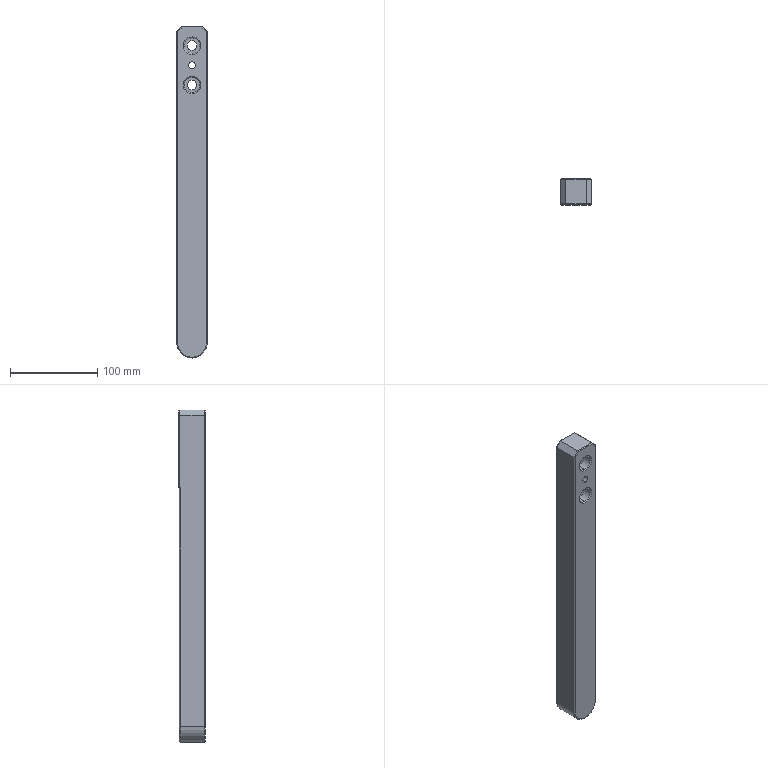Part | Creo | 1 solid | 44 faces | box 35 x 30 x 380 mm | volume 377331 mm3 | plane 23 | cylinder 11 | cone 10 | commonest cylinder face diameters 11 x4 18 x4 8 x2 35 x1
STEP:
#1=CARTESIAN_POINT('',(0.,0.,0.));
#2=DIRECTION('',(0.,0.,1.));
#3=DIRECTION('',(1.,0.,0.));
#4=AXIS2_PLACEMENT_3D('',#1,#2,#3);
#5=CARTESIAN_POINT('',(129.,-219.,0.5));
#6=VERTEX_POINT('',#5);
#7=CARTESIAN_POINT('',(130.,-220.,0.5));
#8=VERTEX_POINT('',#7);
#9=CARTESIAN_POINT('',(129.,-219.,0.5));
#10=DIRECTION('',(0.7071,-0.7071,0.));
#11=VECTOR('',#10,1.414);
#12=LINE('',#9,#11);
#13=EDGE_CURVE('',#6,#8,#12,.T.);
#14=ORIENTED_EDGE('',*,*,#13,.F.);
#15=CARTESIAN_POINT('',(96.,-219.,0.5));
#16=VERTEX_POINT('',#15);
#17=CARTESIAN_POINT('',(129.,-219.,0.5));
#18=DIRECTION('',(-1.,0.,0.));
#19=VECTOR('',#18,33.);
#20=LINE('',#17,#19);
#21=EDGE_CURVE('',#6,#16,#20,.T.);
#22=ORIENTED_EDGE('',*,*,#21,.T.);
#23=CARTESIAN_POINT('',(95.,-220.,0.5));
#24=VERTEX_POINT('',#23);
#25=CARTESIAN_POINT('',(95.,-220.,0.5));
#26=DIRECTION('',(0.7071,0.7071,0.));
#27=VECTOR('',#26,1.414);
#28=LINE('',#25,#27);
#29=EDGE_CURVE('',#24,#16,#28,.T.);
#30=ORIENTED_EDGE('',*,*,#29,.F.);
#31=CARTESIAN_POINT('',(95.,-220.5,0.5));
#32=VERTEX_POINT('',#31);
#33=CARTESIAN_POINT('',(95.,-220.,0.5));
#34=DIRECTION('',(0.,-1.,0.));
#35=VECTOR('',#34,0.5);
#36=LINE('',#33,#35);
#37=EDGE_CURVE('',#24,#32,#36,.T.);
#38=ORIENTED_EDGE('',*,*,#37,.T.);
#39=CARTESIAN_POINT('',(96.,-219.5,0.5));
#40=VERTEX_POINT('',#39);
#41=CARTESIAN_POINT('',(96.,-219.5,0.5));
#42=DIRECTION('',(-0.7071,-0.7071,0.));
#43=VECTOR('',#42,1.414);
#44=LINE('',#41,#43);
#45=EDGE_CURVE('',#40,#32,#44,.T.);
#46=ORIENTED_EDGE('',*,*,#45,.F.);
#47=CARTESIAN_POINT('',(129.,-219.5,0.5));
#48=VERTEX_POINT('',#47);
#49=CARTESIAN_POINT('',(96.,-219.5,0.5));
#50=DIRECTION('',(1.,0.,0.));
#51=VECTOR('',#50,33.);
#52=LINE('',#49,#51);
#53=EDGE_CURVE('',#40,#48,#52,.T.);
#54=ORIENTED_EDGE('',*,*,#53,.T.);
#55=CARTESIAN_POINT('',(130.,-220.5,0.5));
#56=VERTEX_POINT('',#55);
#57=CARTESIAN_POINT('',(130.,-220.5,0.5));
#58=DIRECTION('',(-0.7071,0.7071,0.));
#59=VECTOR('',#58,1.414);
#60=LINE('',#57,#59);
#61=EDGE_CURVE('',#56,#48,#60,.T.);
#62=ORIENTED_EDGE('',*,*,#61,.F.);
#63=CARTESIAN_POINT('',(130.,-220.,0.5));
#64=DIRECTION('',(0.,-1.,0.));
#65=VECTOR('',#64,0.5);
#66=LINE('',#63,#65);
#67=EDGE_CURVE('',#8,#56,#66,.T.);
#68=ORIENTED_EDGE('',*,*,#67,.F.);
#69=EDGE_LOOP('',(#14,#22,#30,#38,#46,#54,#62,#68));
#70=FACE_OUTER_BOUND('',#69,.F.);
#71=CARTESIAN_POINT('',(0.,-7.,0.5));
#72=DIRECTION('',(0.,0.,-1.));
#73=DIRECTION('',(1.,0.,0.));
#74=AXIS2_PLACEMENT_3D('',#71,#72,#73);
#75=PLANE('',#74);
#76=ADVANCED_FACE('',(#70),#75,.T.);
#77=CARTESIAN_POINT('',(130.,-220.,83.5));
#78=VERTEX_POINT('',#77);
#79=CARTESIAN_POINT('',(130.,-220.,83.5));
#80=DIRECTION('',(0.,0.,-1.));
#81=VECTOR('',#80,83.);
#82=LINE('',#79,#81);
#83=EDGE_CURVE('',#78,#8,#82,.T.);
#84=ORIENTED_EDGE('',*,*,#83,.F.);
#85=CARTESIAN_POINT('',(129.,-219.,83.086));
#86=VERTEX_POINT('',#85);
#87=CARTESIAN_POINT('',(129.,-219.,83.086));
#88=DIRECTION('',(0.6786,-0.6786,0.2811));
#89=VECTOR('',#88,1.474);
#90=LINE('',#87,#89);
#91=EDGE_CURVE('',#86,#78,#90,.T.);
#92=ORIENTED_EDGE('',*,*,#91,.F.);
#93=CARTESIAN_POINT('',(129.,-219.,0.5));
#94=DIRECTION('',(0.,0.,1.));
#95=VECTOR('',#94,82.586);
#96=LINE('',#93,#95);
#97=EDGE_CURVE('',#6,#86,#96,.T.);
#98=ORIENTED_EDGE('',*,*,#97,.F.);
#99=ORIENTED_EDGE('',*,*,#13,.T.);
#100=EDGE_LOOP('',(#84,#92,#98,#99));
#101=FACE_OUTER_BOUND('',#100,.F.);
#102=CARTESIAN_POINT('',(129.,-219.,0.));
#103=DIRECTION('',(-0.7071,-0.7071,0.));
#104=DIRECTION('',(0.,0.,-1.));
#105=AXIS2_PLACEMENT_3D('',#102,#103,#104);
#106=PLANE('',#105);
#107=ADVANCED_FACE('',(#101),#106,.F.);
#108=CARTESIAN_POINT('',(130.,-220.5,-273.));
#109=VERTEX_POINT('',#108);
#110=CARTESIAN_POINT('',(130.,-248.,-273.));
#111=VERTEX_POINT('',#110);
#112=CARTESIAN_POINT('',(130.,-220.5,-273.));
#113=DIRECTION('',(0.,-1.,0.));
#114=VECTOR('',#113,27.5);
#115=LINE('',#112,#114);
#116=EDGE_CURVE('',#109,#111,#115,.T.);
#117=ORIENTED_EDGE('',*,*,#116,.T.);
#118=CARTESIAN_POINT('',(130.,-248.,83.5));
#119=VERTEX_POINT('',#118);
#120=CARTESIAN_POINT('',(130.,-248.,-273.));
#121=DIRECTION('',(0.,0.,1.));
#122=VECTOR('',#121,356.5);
#123=LINE('',#120,#122);
#124=EDGE_CURVE('',#111,#119,#123,.T.);
#125=ORIENTED_EDGE('',*,*,#124,.T.);
#126=CARTESIAN_POINT('',(130.,-248.,83.5));
#127=DIRECTION('',(0.,1.,0.));
#128=VECTOR('',#127,28.);
#129=LINE('',#126,#128);
#130=EDGE_CURVE('',#119,#78,#129,.T.);
#131=ORIENTED_EDGE('',*,*,#130,.T.);
#132=ORIENTED_EDGE('',*,*,#83,.T.);
#133=ORIENTED_EDGE('',*,*,#67,.T.);
#134=CARTESIAN_POINT('',(130.,-220.5,0.5));
#135=DIRECTION('',(0.,0.,-1.));
#136=VECTOR('',#135,273.5);
#137=LINE('',#134,#136);
#138=EDGE_CURVE('',#56,#109,#137,.T.);
#139=ORIENTED_EDGE('',*,*,#138,.T.);
#140=EDGE_LOOP('',(#117,#125,#131,#132,#133,#139));
#141=FACE_OUTER_BOUND('',#140,.F.);
#142=CARTESIAN_POINT('',(130.,-249.,79.5));
#143=DIRECTION('',(1.,0.,0.));
#144=DIRECTION('',(0.,0.,-1.));
#145=AXIS2_PLACEMENT_3D('',#142,#143,#144);
#146=PLANE('',#145);
#147=ADVANCED_FACE('',(#141),#146,.T.);
#148=CARTESIAN_POINT('',(95.,-248.,-273.));
#149=VERTEX_POINT('',#148);
#150=CARTESIAN_POINT('',(95.,-220.5,-273.));
#151=VERTEX_POINT('',#150);
#152=CARTESIAN_POINT('',(95.,-248.,-273.));
#153=DIRECTION('',(0.,1.,0.));
#154=VECTOR('',#153,27.5);
#155=LINE('',#152,#154);
#156=EDGE_CURVE('',#149,#151,#155,.T.);
#157=ORIENTED_EDGE('',*,*,#156,.F.);
#158=CARTESIAN_POINT('',(112.5,-248.,-290.5));
#159=VERTEX_POINT('',#158);
#160=CARTESIAN_POINT('',(112.5,-248.,-273.));
#161=DIRECTION('',(0.,-1.,0.));
#162=DIRECTION('',(-1.,0.,0.));
#163=AXIS2_PLACEMENT_3D('',#160,#161,#162);
#164=CIRCLE('',#163,17.5);
#165=EDGE_CURVE('',#149,#159,#164,.T.);
#166=ORIENTED_EDGE('',*,*,#165,.T.);
#167=CARTESIAN_POINT('',(112.5,-248.,-273.));
#168=DIRECTION('',(0.,-1.,0.));
#169=DIRECTION('',(0.,0.,-1.));
#170=AXIS2_PLACEMENT_3D('',#167,#168,#169);
#171=CIRCLE('',#170,17.5);
#172=EDGE_CURVE('',#159,#111,#171,.T.);
#173=ORIENTED_EDGE('',*,*,#172,.T.);
#174=ORIENTED_EDGE('',*,*,#116,.F.);
#175=CARTESIAN_POINT('',(112.5,-220.5,-290.5));
#176=VERTEX_POINT('',#175);
#177=CARTESIAN_POINT('',(112.5,-220.5,-273.));
#178=DIRECTION('',(0.,1.,0.));
#179=DIRECTION('',(1.,0.,0.));
#180=AXIS2_PLACEMENT_3D('',#177,#178,#179);
#181=CIRCLE('',#180,17.5);
#182=EDGE_CURVE('',#109,#176,#181,.T.);
#183=ORIENTED_EDGE('',*,*,#182,.T.);
#184=CARTESIAN_POINT('',(112.5,-220.5,-273.));
#185=DIRECTION('',(0.,1.,0.));
#186=DIRECTION('',(0.,0.,-1.));
#187=AXIS2_PLACEMENT_3D('',#184,#185,#186);
#188=CIRCLE('',#187,17.5);
#189=EDGE_CURVE('',#176,#151,#188,.T.);
#190=ORIENTED_EDGE('',*,*,#189,.T.);
#191=EDGE_LOOP('',(#157,#166,#173,#174,#183,#190));
#192=FACE_OUTER_BOUND('',#191,.F.);
#193=CARTESIAN_POINT('',(112.5,-249.,-273.));
#194=DIRECTION('',(0.,1.,0.));
#195=DIRECTION('',(0.,0.,-1.));
#196=AXIS2_PLACEMENT_3D('',#193,#194,#195);
#197=CYLINDRICAL_SURFACE('',#196,17.5);
#198=ADVANCED_FACE('',(#192),#197,.T.);
#199=CARTESIAN_POINT('',(95.,-220.,83.5));
#200=VERTEX_POINT('',#199);
#201=CARTESIAN_POINT('',(95.,-220.,0.5));
#202=DIRECTION('',(0.,0.,1.));
#203=VECTOR('',#202,83.);
#204=LINE('',#201,#203);
#205=EDGE_CURVE('',#24,#200,#204,.T.);
#206=ORIENTED_EDGE('',*,*,#205,.T.);
#207=CARTESIAN_POINT('',(95.,-248.,83.5));
#208=VERTEX_POINT('',#207);
#209=CARTESIAN_POINT('',(95.,-220.,83.5));
#210=DIRECTION('',(0.,-1.,0.));
#211=VECTOR('',#210,28.);
#212=LINE('',#209,#211);
#213=EDGE_CURVE('',#200,#208,#212,.T.);
#214=ORIENTED_EDGE('',*,*,#213,.T.);
#215=CARTESIAN_POINT('',(95.,-248.,83.5));
#216=DIRECTION('',(0.,0.,-1.));
#217=VECTOR('',#216,356.5);
#218=LINE('',#215,#217);
#219=EDGE_CURVE('',#208,#149,#218,.T.);
#220=ORIENTED_EDGE('',*,*,#219,.T.);
#221=ORIENTED_EDGE('',*,*,#156,.T.);
#222=CARTESIAN_POINT('',(95.,-220.5,-273.));
#223=DIRECTION('',(0.,0.,1.));
#224=VECTOR('',#223,273.5);
#225=LINE('',#222,#224);
#226=EDGE_CURVE('',#151,#32,#225,.T.);
#227=ORIENTED_EDGE('',*,*,#226,.T.);
#228=ORIENTED_EDGE('',*,*,#37,.F.);
#229=EDGE_LOOP('',(#206,#214,#220,#221,#227,#228));
#230=FACE_OUTER_BOUND('',#229,.F.);
#231=CARTESIAN_POINT('',(95.,-249.,-320.5));
#232=DIRECTION('',(-1.,0.,0.));
#233=DIRECTION('',(0.,0.,1.));
#234=AXIS2_PLACEMENT_3D('',#231,#232,#233);
#235=PLANE('',#234);
#236=ADVANCED_FACE('',(#230),#235,.T.);
#237=ORIENTED_EDGE('',*,*,#29,.T.);
#238=CARTESIAN_POINT('',(96.,-219.,83.086));
#239=VERTEX_POINT('',#238);
#240=CARTESIAN_POINT('',(96.,-219.,83.086));
#241=DIRECTION('',(0.,0.,-1.));
#242=VECTOR('',#241,82.586);
#243=LINE('',#240,#242);
#244=EDGE_CURVE('',#239,#16,#243,.T.);
#245=ORIENTED_EDGE('',*,*,#244,.F.);
#246=CARTESIAN_POINT('',(96.,-219.,83.086));
#247=DIRECTION('',(-0.6786,-0.6786,0.2811));
#248=VECTOR('',#247,1.474);
#249=LINE('',#246,#248);
#250=EDGE_CURVE('',#239,#200,#249,.T.);
#251=ORIENTED_EDGE('',*,*,#250,.T.);
#252=ORIENTED_EDGE('',*,*,#205,.F.);
#253=EDGE_LOOP('',(#237,#245,#251,#252));
#254=FACE_OUTER_BOUND('',#253,.F.);
#255=CARTESIAN_POINT('',(96.,-219.,0.));
#256=DIRECTION('',(0.7071,-0.7071,0.));
#257=DIRECTION('',(0.,0.,1.));
#258=AXIS2_PLACEMENT_3D('',#255,#256,#257);
#259=PLANE('',#258);
#260=ADVANCED_FACE('',(#254),#259,.F.);
#261=ORIENTED_EDGE('',*,*,#21,.F.);
#262=ORIENTED_EDGE('',*,*,#97,.T.);
#263=CARTESIAN_POINT('',(123.586,-219.,88.5));
#264=VERTEX_POINT('',#263);
#265=CARTESIAN_POINT('',(123.586,-219.,88.5));
#266=DIRECTION('',(0.7071,0.,-0.7071));
#267=VECTOR('',#266,7.657);
#268=LINE('',#265,#267);
#269=EDGE_CURVE('',#264,#86,#268,.T.);
#270=ORIENTED_EDGE('',*,*,#269,.F.);
#271=CARTESIAN_POINT('',(101.414,-219.,88.5));
#272=VERTEX_POINT('',#271);
#273=CARTESIAN_POINT('',(123.586,-219.,88.5));
#274=DIRECTION('',(-1.,0.,0.));
#275=VECTOR('',#274,22.172);
#276=LINE('',#273,#275);
#277=EDGE_CURVE('',#264,#272,#276,.T.);
#278=ORIENTED_EDGE('',*,*,#277,.T.);
#279=CARTESIAN_POINT('',(96.,-219.,83.086));
#280=DIRECTION('',(0.7071,0.,0.7071));
#281=VECTOR('',#280,7.657);
#282=LINE('',#279,#281);
#283=EDGE_CURVE('',#239,#272,#282,.T.);
#284=ORIENTED_EDGE('',*,*,#283,.F.);
#285=ORIENTED_EDGE('',*,*,#244,.T.);
#286=EDGE_LOOP('',(#261,#262,#270,#278,#284,#285));
#287=FACE_OUTER_BOUND('',#286,.F.);
#288=CARTESIAN_POINT('',(112.5,-219.,15.5));
#289=VERTEX_POINT('',#288);
#290=CARTESIAN_POINT('',(112.5,-219.,28.5));
#291=VERTEX_POINT('',#290);
#292=CARTESIAN_POINT('',(112.5,-219.,22.));
#293=DIRECTION('',(0.,-1.,0.));
#294=DIRECTION('',(0.,0.,-1.));
#295=AXIS2_PLACEMENT_3D('',#292,#293,#294);
#296=CIRCLE('',#295,6.5);
#297=EDGE_CURVE('',#289,#291,#296,.T.);
#298=ORIENTED_EDGE('',*,*,#297,.F.);
#299=CARTESIAN_POINT('',(112.5,-219.,22.));
#300=DIRECTION('',(0.,-1.,0.));
#301=DIRECTION('',(0.,0.,1.));
#302=AXIS2_PLACEMENT_3D('',#299,#300,#301);
#303=CIRCLE('',#302,6.5);
#304=EDGE_CURVE('',#291,#289,#303,.T.);
#305=ORIENTED_EDGE('',*,*,#304,.F.);
#306=EDGE_LOOP('',(#298,#305));
#307=FACE_BOUND('',#306,.F.);
#308=CARTESIAN_POINT('',(112.5,-219.,60.5));
#309=VERTEX_POINT('',#308);
#310=CARTESIAN_POINT('',(112.5,-219.,73.5));
#311=VERTEX_POINT('',#310);
#312=CARTESIAN_POINT('',(112.5,-219.,67.));
#313=DIRECTION('',(0.,-1.,0.));
#314=DIRECTION('',(0.,0.,-1.));
#315=AXIS2_PLACEMENT_3D('',#312,#313,#314);
#316=CIRCLE('',#315,6.5);
#317=EDGE_CURVE('',#309,#311,#316,.T.);
#318=ORIENTED_EDGE('',*,*,#317,.F.);
#319=CARTESIAN_POINT('',(112.5,-219.,67.));
#320=DIRECTION('',(0.,-1.,0.));
#321=DIRECTION('',(0.,0.,1.));
#322=AXIS2_PLACEMENT_3D('',#319,#320,#321);
#323=CIRCLE('',#322,6.5);
#324=EDGE_CURVE('',#311,#309,#323,.T.);
#325=ORIENTED_EDGE('',*,*,#324,.F.);
#326=EDGE_LOOP('',(#318,#325));
#327=FACE_BOUND('',#326,.F.);
#328=CARTESIAN_POINT('',(112.5,-219.,40.5));
#329=VERTEX_POINT('',#328);
#330=CARTESIAN_POINT('',(112.5,-219.,48.5));
#331=VERTEX_POINT('',#330);
#332=CARTESIAN_POINT('',(112.5,-219.,44.5));
#333=DIRECTION('',(0.,-1.,0.));
#334=DIRECTION('',(0.,0.,-1.));
#335=AXIS2_PLACEMENT_3D('',#332,#333,#334);
#336=CIRCLE('',#335,4.);
#337=EDGE_CURVE('',#329,#331,#336,.T.);
#338=ORIENTED_EDGE('',*,*,#337,.F.);
#339=CARTESIAN_POINT('',(112.5,-219.,44.5));
#340=DIRECTION('',(0.,-1.,0.));
#341=DIRECTION('',(0.,0.,1.));
#342=AXIS2_PLACEMENT_3D('',#339,#340,#341);
#343=CIRCLE('',#342,4.);
#344=EDGE_CURVE('',#331,#329,#343,.T.);
#345=ORIENTED_EDGE('',*,*,#344,.F.);
#346=EDGE_LOOP('',(#338,#345));
#347=FACE_BOUND('',#346,.F.);
#348=CARTESIAN_POINT('',(0.,-219.,0.));
#349=DIRECTION('',(0.,1.,0.));
#350=DIRECTION('',(0.,0.,1.));
#351=AXIS2_PLACEMENT_3D('',#348,#349,#350);
#352=PLANE('',#351);
#353=ADVANCED_FACE('',(#287,#307,#327,#347),#352,.T.);
#354=ORIENTED_EDGE('',*,*,#337,.T.);
#355=CARTESIAN_POINT('',(112.5,-249.,48.5));
#356=VERTEX_POINT('',#355);
#357=CARTESIAN_POINT('',(112.5,-249.,48.5));
#358=DIRECTION('',(0.,1.,0.));
#359=VECTOR('',#358,30.);
#360=LINE('',#357,#359);
#361=EDGE_CURVE('',#356,#331,#360,.T.);
#362=ORIENTED_EDGE('',*,*,#361,.F.);
#363=CARTESIAN_POINT('',(112.5,-249.,40.5));
#364=VERTEX_POINT('',#363);
#365=CARTESIAN_POINT('',(112.5,-249.,44.5));
#366=DIRECTION('',(0.,1.,0.));
#367=DIRECTION('',(0.,0.,1.));
#368=AXIS2_PLACEMENT_3D('',#365,#366,#367);
#369=CIRCLE('',#368,4.);
#370=EDGE_CURVE('',#356,#364,#369,.T.);
#371=ORIENTED_EDGE('',*,*,#370,.T.);
#372=CARTESIAN_POINT('',(112.5,-249.,40.5));
#373=DIRECTION('',(0.,1.,0.));
#374=VECTOR('',#373,30.);
#375=LINE('',#372,#374);
#376=EDGE_CURVE('',#364,#329,#375,.T.);
#377=ORIENTED_EDGE('',*,*,#376,.T.);
#378=EDGE_LOOP('',(#354,#362,#371,#377));
#379=FACE_OUTER_BOUND('',#378,.F.);
#380=CARTESIAN_POINT('',(112.5,-249.,44.5));
#381=DIRECTION('',(0.,1.,0.));
#382=DIRECTION('',(0.,0.,-1.));
#383=AXIS2_PLACEMENT_3D('',#380,#381,#382);
#384=CYLINDRICAL_SURFACE('',#383,4.);
#385=ADVANCED_FACE('',(#379),#384,.F.);
#386=ORIENTED_EDGE('',*,*,#344,.T.);
#387=ORIENTED_EDGE('',*,*,#376,.F.);
#388=CARTESIAN_POINT('',(112.5,-249.,44.5));
#389=DIRECTION('',(0.,1.,0.));
#390=DIRECTION('',(0.,0.,-1.));
#391=AXIS2_PLACEMENT_3D('',#388,#389,#390);
#392=CIRCLE('',#391,4.);
#393=EDGE_CURVE('',#364,#356,#392,.T.);
#394=ORIENTED_EDGE('',*,*,#393,.T.);
#395=ORIENTED_EDGE('',*,*,#361,.T.);
#396=EDGE_LOOP('',(#386,#387,#394,#395));
#397=FACE_OUTER_BOUND('',#396,.F.);
#398=CARTESIAN_POINT('',(112.5,-249.,44.5));
#399=DIRECTION('',(0.,1.,0.));
#400=DIRECTION('',(0.,0.,-1.));
#401=AXIS2_PLACEMENT_3D('',#398,#399,#400);
#402=CYLINDRICAL_SURFACE('',#401,4.);
#403=ADVANCED_FACE('',(#397),#402,.F.);
#404=CARTESIAN_POINT('',(101.414,-249.,88.5));
#405=VERTEX_POINT('',#404);
#406=CARTESIAN_POINT('',(123.586,-249.,88.5));
#407=VERTEX_POINT('',#406);
#408=CARTESIAN_POINT('',(101.414,-249.,88.5));
#409=DIRECTION('',(1.,0.,0.));
#410=VECTOR('',#409,22.172);
#411=LINE('',#408,#410);
#412=EDGE_CURVE('',#405,#407,#411,.T.);
#413=ORIENTED_EDGE('',*,*,#412,.T.);
#414=CARTESIAN_POINT('',(129.,-249.,83.086));
#415=VERTEX_POINT('',#414);
#416=CARTESIAN_POINT('',(129.,-249.,83.086));
#417=DIRECTION('',(-0.7071,0.,0.7071));
#418=VECTOR('',#417,7.657);
#419=LINE('',#416,#418);
#420=EDGE_CURVE('',#415,#407,#419,.T.);
#421=ORIENTED_EDGE('',*,*,#420,.F.);
#422=CARTESIAN_POINT('',(129.,-249.,-273.));
#423=VERTEX_POINT('',#422);
#424=CARTESIAN_POINT('',(129.,-249.,83.086));
#425=DIRECTION('',(0.,0.,-1.));
#426=VECTOR('',#425,356.086);
#427=LINE('',#424,#426);
#428=EDGE_CURVE('',#415,#423,#427,.T.);
#429=ORIENTED_EDGE('',*,*,#428,.T.);
#430=CARTESIAN_POINT('',(96.,-249.,-273.));
#431=VERTEX_POINT('',#430);
#432=CARTESIAN_POINT('',(112.5,-249.,-273.));
#433=DIRECTION('',(0.,-1.,0.));
#434=DIRECTION('',(-1.,0.,0.));
#435=AXIS2_PLACEMENT_3D('',#432,#433,#434);
#436=CIRCLE('',#435,16.5);
#437=EDGE_CURVE('',#431,#423,#436,.T.);
#438=ORIENTED_EDGE('',*,*,#437,.F.);
#439=CARTESIAN_POINT('',(96.,-249.,83.086));
#440=VERTEX_POINT('',#439);
#441=CARTESIAN_POINT('',(96.,-249.,-273.));
#442=DIRECTION('',(0.,0.,1.));
#443=VECTOR('',#442,356.086);
#444=LINE('',#441,#443);
#445=EDGE_CURVE('',#431,#440,#444,.T.);
#446=ORIENTED_EDGE('',*,*,#445,.T.);
#447=CARTESIAN_POINT('',(101.414,-249.,88.5));
#448=DIRECTION('',(-0.7071,0.,-0.7071));
#449=VECTOR('',#448,7.657);
#450=LINE('',#447,#449);
#451=EDGE_CURVE('',#405,#440,#450,.T.);
#452=ORIENTED_EDGE('',*,*,#451,.F.);
#453=EDGE_LOOP('',(#413,#421,#429,#438,#446,#452));
#454=FACE_OUTER_BOUND('',#453,.F.);
#455=CARTESIAN_POINT('',(112.5,-249.,12.));
#456=VERTEX_POINT('',#455);
#457=CARTESIAN_POINT('',(112.5,-249.,32.));
#458=VERTEX_POINT('',#457);
#459=CARTESIAN_POINT('',(112.5,-249.,22.));
#460=DIRECTION('',(0.,1.,0.));
#461=DIRECTION('',(0.,0.,-1.));
#462=AXIS2_PLACEMENT_3D('',#459,#460,#461);
#463=CIRCLE('',#462,10.);
#464=EDGE_CURVE('',#456,#458,#463,.T.);
#465=ORIENTED_EDGE('',*,*,#464,.F.);
#466=CARTESIAN_POINT('',(112.5,-249.,22.));
#467=DIRECTION('',(0.,1.,0.));
#468=DIRECTION('',(0.,0.,1.));
#469=AXIS2_PLACEMENT_3D('',#466,#467,#468);
#470=CIRCLE('',#469,10.);
#471=EDGE_CURVE('',#458,#456,#470,.T.);
#472=ORIENTED_EDGE('',*,*,#471,.F.);
#473=EDGE_LOOP('',(#465,#472));
#474=FACE_BOUND('',#473,.F.);
#475=CARTESIAN_POINT('',(112.5,-249.,57.));
#476=VERTEX_POINT('',#475);
#477=CARTESIAN_POINT('',(112.5,-249.,77.));
#478=VERTEX_POINT('',#477);
#479=CARTESIAN_POINT('',(112.5,-249.,67.));
#480=DIRECTION('',(0.,1.,0.));
#481=DIRECTION('',(0.,0.,-1.));
#482=AXIS2_PLACEMENT_3D('',#479,#480,#481);
#483=CIRCLE('',#482,10.);
#484=EDGE_CURVE('',#476,#478,#483,.T.);
#485=ORIENTED_EDGE('',*,*,#484,.F.);
#486=CARTESIAN_POINT('',(112.5,-249.,67.));
#487=DIRECTION('',(0.,1.,0.));
#488=DIRECTION('',(0.,0.,1.));
#489=AXIS2_PLACEMENT_3D('',#486,#487,#488);
#490=CIRCLE('',#489,10.);
#491=EDGE_CURVE('',#478,#476,#490,.T.);
#492=ORIENTED_EDGE('',*,*,#491,.F.);
#493=EDGE_LOOP('',(#485,#492));
#494=FACE_BOUND('',#493,.F.);
#495=ORIENTED_EDGE('',*,*,#393,.F.);
#496=ORIENTED_EDGE('',*,*,#370,.F.);
#497=EDGE_LOOP('',(#495,#496));
#498=FACE_BOUND('',#497,.F.);
#499=CARTESIAN_POINT('',(0.,-249.,0.));
#500=DIRECTION('',(0.,1.,0.));
#501=DIRECTION('',(0.,0.,1.));
#502=AXIS2_PLACEMENT_3D('',#499,#500,#501);
#503=PLANE('',#502);
#504=ADVANCED_FACE('',(#454,#474,#494,#498),#503,.F.);
#505=CARTESIAN_POINT('',(112.5,-248.,13.));
#506=VERTEX_POINT('',#505);
#507=CARTESIAN_POINT('',(112.5,-248.,31.));
#508=VERTEX_POINT('',#507);
#509=CARTESIAN_POINT('',(112.5,-248.,22.));
#510=DIRECTION('',(0.,1.,0.));
#511=DIRECTION('',(0.,0.,-1.));
#512=AXIS2_PLACEMENT_3D('',#509,#510,#511);
#513=CIRCLE('',#512,9.);
#514=EDGE_CURVE('',#506,#508,#513,.T.);
#515=ORIENTED_EDGE('',*,*,#514,.F.);
#516=CARTESIAN_POINT('',(112.5,-248.,13.));
#517=DIRECTION('',(0.,-0.7071,-0.7071));
#518=VECTOR('',#517,1.414);
#519=LINE('',#516,#518);
#520=EDGE_CURVE('',#506,#456,#519,.T.);
#521=ORIENTED_EDGE('',*,*,#520,.T.);
#522=ORIENTED_EDGE('',*,*,#464,.T.);
#523=CARTESIAN_POINT('',(112.5,-248.,31.));
#524=DIRECTION('',(0.,-0.7071,0.7071));
#525=VECTOR('',#524,1.414);
#526=LINE('',#523,#525);
#527=EDGE_CURVE('',#508,#458,#526,.T.);
#528=ORIENTED_EDGE('',*,*,#527,.F.);
#529=EDGE_LOOP('',(#515,#521,#522,#528));
#530=FACE_OUTER_BOUND('',#529,.F.);
#531=CARTESIAN_POINT('',(112.5,-248.5,22.));
#532=DIRECTION('',(0.,-1.,0.));
#533=DIRECTION('',(0.,0.,1.));
#534=AXIS2_PLACEMENT_3D('',#531,#532,#533);
#535=CONICAL_SURFACE('',#534,9.5,45.);
#536=ADVANCED_FACE('',(#530),#535,.F.);
#537=ORIENTED_EDGE('',*,*,#514,.T.);
#538=CARTESIAN_POINT('',(112.5,-238.,31.));
#539=VERTEX_POINT('',#538);
#540=CARTESIAN_POINT('',(112.5,-248.,31.));
#541=DIRECTION('',(0.,1.,0.));
#542=VECTOR('',#541,10.);
#543=LINE('',#540,#542);
#544=EDGE_CURVE('',#508,#539,#543,.T.);
#545=ORIENTED_EDGE('',*,*,#544,.T.);
#546=CARTESIAN_POINT('',(112.5,-238.,13.));
#547=VERTEX_POINT('',#546);
#548=CARTESIAN_POINT('',(112.5,-238.,22.));
#549=DIRECTION('',(0.,-1.,0.));
#550=DIRECTION('',(0.,0.,1.));
#551=AXIS2_PLACEMENT_3D('',#548,#549,#550);
#552=CIRCLE('',#551,9.);
#553=EDGE_CURVE('',#539,#547,#552,.T.);
#554=ORIENTED_EDGE('',*,*,#553,.T.);
#555=CARTESIAN_POINT('',(112.5,-248.,13.));
#556=DIRECTION('',(0.,1.,0.));
#557=VECTOR('',#556,10.);
#558=LINE('',#555,#557);
#559=EDGE_CURVE('',#506,#547,#558,.T.);
#560=ORIENTED_EDGE('',*,*,#559,.F.);
#561=EDGE_LOOP('',(#537,#545,#554,#560));
#562=FACE_OUTER_BOUND('',#561,.F.);
#563=CARTESIAN_POINT('',(112.5,-249.,22.));
#564=DIRECTION('',(0.,1.,0.));
#565=DIRECTION('',(0.,0.,-1.));
#566=AXIS2_PLACEMENT_3D('',#563,#564,#565);
#567=CYLINDRICAL_SURFACE('',#566,9.);
#568=ADVANCED_FACE('',(#562),#567,.F.);
#569=CARTESIAN_POINT('',(112.5,-248.,22.));
#570=DIRECTION('',(0.,1.,0.));
#571=DIRECTION('',(0.,0.,1.));
#572=AXIS2_PLACEMENT_3D('',#569,#570,#571);
#573=CIRCLE('',#572,9.);
#574=EDGE_CURVE('',#508,#506,#573,.T.);
#575=ORIENTED_EDGE('',*,*,#574,.T.);
#576=ORIENTED_EDGE('',*,*,#559,.T.);
#577=CARTESIAN_POINT('',(112.5,-238.,22.));
#578=DIRECTION('',(0.,-1.,0.));
#579=DIRECTION('',(0.,0.,-1.));
#580=AXIS2_PLACEMENT_3D('',#577,#578,#579);
#581=CIRCLE('',#580,9.);
#582=EDGE_CURVE('',#547,#539,#581,.T.);
#583=ORIENTED_EDGE('',*,*,#582,.T.);
#584=ORIENTED_EDGE('',*,*,#544,.F.);
#585=EDGE_LOOP('',(#575,#576,#583,#584));
#586=FACE_OUTER_BOUND('',#585,.F.);
#587=CARTESIAN_POINT('',(112.5,-249.,22.));
#588=DIRECTION('',(0.,1.,0.));
#589=DIRECTION('',(0.,0.,-1.));
#590=AXIS2_PLACEMENT_3D('',#587,#588,#589);
#591=CYLINDRICAL_SURFACE('',#590,9.);
#592=ADVANCED_FACE('',(#586),#591,.F.);
#593=ORIENTED_EDGE('',*,*,#574,.F.);
#594=ORIENTED_EDGE('',*,*,#527,.T.);
#595=ORIENTED_EDGE('',*,*,#471,.T.);
#596=ORIENTED_EDGE('',*,*,#520,.F.);
#597=EDGE_LOOP('',(#593,#594,#595,#596));
#598=FACE_OUTER_BOUND('',#597,.F.);
#599=CARTESIAN_POINT('',(112.5,-248.5,22.));
#600=DIRECTION('',(0.,-1.,0.));
#601=DIRECTION('',(0.,0.,1.));
#602=AXIS2_PLACEMENT_3D('',#599,#600,#601);
#603=CONICAL_SURFACE('',#602,9.5,45.);
#604=ADVANCED_FACE('',(#598),#603,.F.);
#605=ORIENTED_EDGE('',*,*,#582,.F.);
#606=ORIENTED_EDGE('',*,*,#553,.F.);
#607=EDGE_LOOP('',(#605,#606));
#608=FACE_OUTER_BOUND('',#607,.F.);
#609=CARTESIAN_POINT('',(112.5,-238.,16.5));
#610=VERTEX_POINT('',#609);
#611=CARTESIAN_POINT('',(112.5,-238.,27.5));
#612=VERTEX_POINT('',#611);
#613=CARTESIAN_POINT('',(112.5,-238.,22.));
#614=DIRECTION('',(0.,1.,0.));
#615=DIRECTION('',(0.,0.,-1.));
#616=AXIS2_PLACEMENT_3D('',#613,#614,#615);
#617=CIRCLE('',#616,5.5);
#618=EDGE_CURVE('',#610,#612,#617,.T.);
#619=ORIENTED_EDGE('',*,*,#618,.F.);
#620=CARTESIAN_POINT('',(112.5,-238.,22.));
#621=DIRECTION('',(0.,1.,0.));
#622=DIRECTION('',(0.,0.,1.));
#623=AXIS2_PLACEMENT_3D('',#620,#621,#622);
#624=CIRCLE('',#623,5.5);
#625=EDGE_CURVE('',#612,#610,#624,.T.);
#626=ORIENTED_EDGE('',*,*,#625,.F.);
#627=EDGE_LOOP('',(#619,#626));
#628=FACE_BOUND('',#627,.F.);
#629=CARTESIAN_POINT('',(112.5,-238.,22.));
#630=DIRECTION('',(0.,1.,0.));
#631=DIRECTION('',(0.,0.,-1.));
#632=AXIS2_PLACEMENT_3D('',#629,#630,#631);
#633=PLANE('',#632);
#634=ADVANCED_FACE('',(#608,#628),#633,.F.);
#635=CARTESIAN_POINT('',(112.5,-220.,27.5));
#636=VERTEX_POINT('',#635);
#637=CARTESIAN_POINT('',(112.5,-220.,16.5));
#638=VERTEX_POINT('',#637);
#639=CARTESIAN_POINT('',(112.5,-220.,22.));
#640=DIRECTION('',(0.,-1.,0.));
#641=DIRECTION('',(0.,0.,1.));
#642=AXIS2_PLACEMENT_3D('',#639,#640,#641);
#643=CIRCLE('',#642,5.5);
#644=EDGE_CURVE('',#636,#638,#643,.T.);
#645=ORIENTED_EDGE('',*,*,#644,.T.);
#646=CARTESIAN_POINT('',(112.5,-238.,16.5));
#647=DIRECTION('',(0.,1.,0.));
#648=VECTOR('',#647,18.);
#649=LINE('',#646,#648);
#650=EDGE_CURVE('',#610,#638,#649,.T.);
#651=ORIENTED_EDGE('',*,*,#650,.F.);
#652=ORIENTED_EDGE('',*,*,#618,.T.);
#653=CARTESIAN_POINT('',(112.5,-238.,27.5));
#654=DIRECTION('',(0.,1.,0.));
#655=VECTOR('',#654,18.);
#656=LINE('',#653,#655);
#657=EDGE_CURVE('',#612,#636,#656,.T.);
#658=ORIENTED_EDGE('',*,*,#657,.T.);
#659=EDGE_LOOP('',(#645,#651,#652,#658));
#660=FACE_OUTER_BOUND('',#659,.F.);
#661=CARTESIAN_POINT('',(112.5,-49.,22.));
#662=DIRECTION('',(0.,1.,0.));
#663=DIRECTION('',(0.,0.,-1.));
#664=AXIS2_PLACEMENT_3D('',#661,#662,#663);
#665=CYLINDRICAL_SURFACE('',#664,5.5);
#666=ADVANCED_FACE('',(#660),#665,.F.);
#667=ORIENTED_EDGE('',*,*,#304,.T.);
#668=CARTESIAN_POINT('',(112.5,-220.,16.5));
#669=DIRECTION('',(0.,0.7071,-0.7071));
#670=VECTOR('',#669,1.414);
#671=LINE('',#668,#670);
#672=EDGE_CURVE('',#638,#289,#671,.T.);
#673=ORIENTED_EDGE('',*,*,#672,.F.);
#674=ORIENTED_EDGE('',*,*,#644,.F.);
#675=CARTESIAN_POINT('',(112.5,-220.,27.5));
#676=DIRECTION('',(0.,0.7071,0.7071));
#677=VECTOR('',#676,1.414);
#678=LINE('',#675,#677);
#679=EDGE_CURVE('',#636,#291,#678,.T.);
#680=ORIENTED_EDGE('',*,*,#679,.T.);
#681=EDGE_LOOP('',(#667,#673,#674,#680));
#682=FACE_OUTER_BOUND('',#681,.F.);
#683=CARTESIAN_POINT('',(112.5,-219.5,22.));
#684=DIRECTION('',(0.,1.,0.));
#685=DIRECTION('',(0.,0.,-1.));
#686=AXIS2_PLACEMENT_3D('',#683,#684,#685);
#687=CONICAL_SURFACE('',#686,6.,45.);
#688=ADVANCED_FACE('',(#682),#687,.F.);
#689=ORIENTED_EDGE('',*,*,#297,.T.);
#690=ORIENTED_EDGE('',*,*,#679,.F.);
#691=CARTESIAN_POINT('',(112.5,-220.,22.));
#692=DIRECTION('',(0.,-1.,0.));
#693=DIRECTION('',(0.,0.,-1.));
#694=AXIS2_PLACEMENT_3D('',#691,#692,#693);
#695=CIRCLE('',#694,5.5);
#696=EDGE_CURVE('',#638,#636,#695,.T.);
#697=ORIENTED_EDGE('',*,*,#696,.F.);
#698=ORIENTED_EDGE('',*,*,#672,.T.);
#699=EDGE_LOOP('',(#689,#690,#697,#698));
#700=FACE_OUTER_BOUND('',#699,.F.);
#701=CARTESIAN_POINT('',(112.5,-219.5,22.));
#702=DIRECTION('',(0.,1.,0.));
#703=DIRECTION('',(0.,0.,-1.));
#704=AXIS2_PLACEMENT_3D('',#701,#702,#703);
#705=CONICAL_SURFACE('',#704,6.,45.);
#706=ADVANCED_FACE('',(#700),#705,.F.);
#707=ORIENTED_EDGE('',*,*,#696,.T.);
#708=ORIENTED_EDGE('',*,*,#657,.F.);
#709=ORIENTED_EDGE('',*,*,#625,.T.);
#710=ORIENTED_EDGE('',*,*,#650,.T.);
#711=EDGE_LOOP('',(#707,#708,#709,#710));
#712=FACE_OUTER_BOUND('',#711,.F.);
#713=CARTESIAN_POINT('',(112.5,-49.,22.));
#714=DIRECTION('',(0.,1.,0.));
#715=DIRECTION('',(0.,0.,-1.));
#716=AXIS2_PLACEMENT_3D('',#713,#714,#715);
#717=CYLINDRICAL_SURFACE('',#716,5.5);
#718=ADVANCED_FACE('',(#712),#717,.F.);
#719=CARTESIAN_POINT('',(112.5,-248.,58.));
#720=VERTEX_POINT('',#719);
#721=CARTESIAN_POINT('',(112.5,-248.,76.));
#722=VERTEX_POINT('',#721);
#723=CARTESIAN_POINT('',(112.5,-248.,67.));
#724=DIRECTION('',(0.,1.,0.));
#725=DIRECTION('',(0.,0.,-1.));
#726=AXIS2_PLACEMENT_3D('',#723,#724,#725);
#727=CIRCLE('',#726,9.);
#728=EDGE_CURVE('',#720,#722,#727,.T.);
#729=ORIENTED_EDGE('',*,*,#728,.F.);
#730=CARTESIAN_POINT('',(112.5,-248.,58.));
#731=DIRECTION('',(0.,-0.7071,-0.7071));
#732=VECTOR('',#731,1.414);
#733=LINE('',#730,#732);
#734=EDGE_CURVE('',#720,#476,#733,.T.);
#735=ORIENTED_EDGE('',*,*,#734,.T.);
#736=ORIENTED_EDGE('',*,*,#484,.T.);
#737=CARTESIAN_POINT('',(112.5,-248.,76.));
#738=DIRECTION('',(0.,-0.7071,0.7071));
#739=VECTOR('',#738,1.414);
#740=LINE('',#737,#739);
#741=EDGE_CURVE('',#722,#478,#740,.T.);
#742=ORIENTED_EDGE('',*,*,#741,.F.);
#743=EDGE_LOOP('',(#729,#735,#736,#742));
#744=FACE_OUTER_BOUND('',#743,.F.);
#745=CARTESIAN_POINT('',(112.5,-248.5,67.));
#746=DIRECTION('',(0.,-1.,0.));
#747=DIRECTION('',(0.,0.,1.));
#748=AXIS2_PLACEMENT_3D('',#745,#746,#747);
#749=CONICAL_SURFACE('',#748,9.5,45.);
#750=ADVANCED_FACE('',(#744),#749,.F.);
#751=ORIENTED_EDGE('',*,*,#728,.T.);
#752=CARTESIAN_POINT('',(112.5,-238.,76.));
#753=VERTEX_POINT('',#752);
#754=CARTESIAN_POINT('',(112.5,-248.,76.));
#755=DIRECTION('',(0.,1.,0.));
#756=VECTOR('',#755,10.);
#757=LINE('',#754,#756);
#758=EDGE_CURVE('',#722,#753,#757,.T.);
#759=ORIENTED_EDGE('',*,*,#758,.T.);
#760=CARTESIAN_POINT('',(112.5,-238.,58.));
#761=VERTEX_POINT('',#760);
#762=CARTESIAN_POINT('',(112.5,-238.,67.));
#763=DIRECTION('',(0.,-1.,0.));
#764=DIRECTION('',(0.,0.,1.));
#765=AXIS2_PLACEMENT_3D('',#762,#763,#764);
#766=CIRCLE('',#765,9.);
#767=EDGE_CURVE('',#753,#761,#766,.T.);
#768=ORIENTED_EDGE('',*,*,#767,.T.);
#769=CARTESIAN_POINT('',(112.5,-248.,58.));
#770=DIRECTION('',(0.,1.,0.));
#771=VECTOR('',#770,10.);
#772=LINE('',#769,#771);
#773=EDGE_CURVE('',#720,#761,#772,.T.);
#774=ORIENTED_EDGE('',*,*,#773,.F.);
#775=EDGE_LOOP('',(#751,#759,#768,#774));
#776=FACE_OUTER_BOUND('',#775,.F.);
#777=CARTESIAN_POINT('',(112.5,-249.,67.));
#778=DIRECTION('',(0.,1.,0.));
#779=DIRECTION('',(0.,0.,-1.));
#780=AXIS2_PLACEMENT_3D('',#777,#778,#779);
#781=CYLINDRICAL_SURFACE('',#780,9.);
#782=ADVANCED_FACE('',(#776),#781,.F.);
#783=CARTESIAN_POINT('',(112.5,-248.,67.));
#784=DIRECTION('',(0.,1.,0.));
#785=DIRECTION('',(0.,0.,1.));
#786=AXIS2_PLACEMENT_3D('',#783,#784,#785);
#787=CIRCLE('',#786,9.);
#788=EDGE_CURVE('',#722,#720,#787,.T.);
#789=ORIENTED_EDGE('',*,*,#788,.T.);
#790=ORIENTED_EDGE('',*,*,#773,.T.);
#791=CARTESIAN_POINT('',(112.5,-238.,67.));
#792=DIRECTION('',(0.,-1.,0.));
#793=DIRECTION('',(0.,0.,-1.));
#794=AXIS2_PLACEMENT_3D('',#791,#792,#793);
#795=CIRCLE('',#794,9.);
#796=EDGE_CURVE('',#761,#753,#795,.T.);
#797=ORIENTED_EDGE('',*,*,#796,.T.);
#798=ORIENTED_EDGE('',*,*,#758,.F.);
#799=EDGE_LOOP('',(#789,#790,#797,#798));
#800=FACE_OUTER_BOUND('',#799,.F.);
#801=CARTESIAN_POINT('',(112.5,-249.,67.));
#802=DIRECTION('',(0.,1.,0.));
#803=DIRECTION('',(0.,0.,-1.));
#804=AXIS2_PLACEMENT_3D('',#801,#802,#803);
#805=CYLINDRICAL_SURFACE('',#804,9.);
#806=ADVANCED_FACE('',(#800),#805,.F.);
#807=ORIENTED_EDGE('',*,*,#788,.F.);
#808=ORIENTED_EDGE('',*,*,#741,.T.);
#809=ORIENTED_EDGE('',*,*,#491,.T.);
#810=ORIENTED_EDGE('',*,*,#734,.F.);
#811=EDGE_LOOP('',(#807,#808,#809,#810));
#812=FACE_OUTER_BOUND('',#811,.F.);
#813=CARTESIAN_POINT('',(112.5,-248.5,67.));
#814=DIRECTION('',(0.,-1.,0.));
#815=DIRECTION('',(0.,0.,1.));
#816=AXIS2_PLACEMENT_3D('',#813,#814,#815);
#817=CONICAL_SURFACE('',#816,9.5,45.);
#818=ADVANCED_FACE('',(#812),#817,.F.);
#819=ORIENTED_EDGE('',*,*,#796,.F.);
#820=ORIENTED_EDGE('',*,*,#767,.F.);
#821=EDGE_LOOP('',(#819,#820));
#822=FACE_OUTER_BOUND('',#821,.F.);
#823=CARTESIAN_POINT('',(112.5,-238.,61.5));
#824=VERTEX_POINT('',#823);
#825=CARTESIAN_POINT('',(112.5,-238.,72.5));
#826=VERTEX_POINT('',#825);
#827=CARTESIAN_POINT('',(112.5,-238.,67.));
#828=DIRECTION('',(0.,1.,0.));
#829=DIRECTION('',(0.,0.,-1.));
#830=AXIS2_PLACEMENT_3D('',#827,#828,#829);
#831=CIRCLE('',#830,5.5);
#832=EDGE_CURVE('',#824,#826,#831,.T.);
#833=ORIENTED_EDGE('',*,*,#832,.F.);
#834=CARTESIAN_POINT('',(112.5,-238.,67.));
#835=DIRECTION('',(0.,1.,0.));
#836=DIRECTION('',(0.,0.,1.));
#837=AXIS2_PLACEMENT_3D('',#834,#835,#836);
#838=CIRCLE('',#837,5.5);
#839=EDGE_CURVE('',#826,#824,#838,.T.);
#840=ORIENTED_EDGE('',*,*,#839,.F.);
#841=EDGE_LOOP('',(#833,#840));
#842=FACE_BOUND('',#841,.F.);
#843=CARTESIAN_POINT('',(112.5,-238.,67.));
#844=DIRECTION('',(0.,1.,0.));
#845=DIRECTION('',(0.,0.,-1.));
#846=AXIS2_PLACEMENT_3D('',#843,#844,#845);
#847=PLANE('',#846);
#848=ADVANCED_FACE('',(#822,#842),#847,.F.);
#849=CARTESIAN_POINT('',(112.5,-220.,72.5));
#850=VERTEX_POINT('',#849);
#851=CARTESIAN_POINT('',(112.5,-220.,61.5));
#852=VERTEX_POINT('',#851);
#853=CARTESIAN_POINT('',(112.5,-220.,67.));
#854=DIRECTION('',(0.,-1.,0.));
#855=DIRECTION('',(0.,0.,1.));
#856=AXIS2_PLACEMENT_3D('',#853,#854,#855);
#857=CIRCLE('',#856,5.5);
#858=EDGE_CURVE('',#850,#852,#857,.T.);
#859=ORIENTED_EDGE('',*,*,#858,.T.);
#860=CARTESIAN_POINT('',(112.5,-238.,61.5));
#861=DIRECTION('',(0.,1.,0.));
#862=VECTOR('',#861,18.);
#863=LINE('',#860,#862);
#864=EDGE_CURVE('',#824,#852,#863,.T.);
#865=ORIENTED_EDGE('',*,*,#864,.F.);
#866=ORIENTED_EDGE('',*,*,#832,.T.);
#867=CARTESIAN_POINT('',(112.5,-238.,72.5));
#868=DIRECTION('',(0.,1.,0.));
#869=VECTOR('',#868,18.);
#870=LINE('',#867,#869);
#871=EDGE_CURVE('',#826,#850,#870,.T.);
#872=ORIENTED_EDGE('',*,*,#871,.T.);
#873=EDGE_LOOP('',(#859,#865,#866,#872));
#874=FACE_OUTER_BOUND('',#873,.F.);
#875=CARTESIAN_POINT('',(112.5,-49.,67.));
#876=DIRECTION('',(0.,1.,0.));
#877=DIRECTION('',(0.,0.,-1.));
#878=AXIS2_PLACEMENT_3D('',#875,#876,#877);
#879=CYLINDRICAL_SURFACE('',#878,5.5);
#880=ADVANCED_FACE('',(#874),#879,.F.);
#881=ORIENTED_EDGE('',*,*,#324,.T.);
#882=CARTESIAN_POINT('',(112.5,-220.,61.5));
#883=DIRECTION('',(0.,0.7071,-0.7071));
#884=VECTOR('',#883,1.414);
#885=LINE('',#882,#884);
#886=EDGE_CURVE('',#852,#309,#885,.T.);
#887=ORIENTED_EDGE('',*,*,#886,.F.);
#888=ORIENTED_EDGE('',*,*,#858,.F.);
#889=CARTESIAN_POINT('',(112.5,-220.,72.5));
#890=DIRECTION('',(0.,0.7071,0.7071));
#891=VECTOR('',#890,1.414);
#892=LINE('',#889,#891);
#893=EDGE_CURVE('',#850,#311,#892,.T.);
#894=ORIENTED_EDGE('',*,*,#893,.T.);
#895=EDGE_LOOP('',(#881,#887,#888,#894));
#896=FACE_OUTER_BOUND('',#895,.F.);
#897=CARTESIAN_POINT('',(112.5,-219.5,67.));
#898=DIRECTION('',(0.,1.,0.));
#899=DIRECTION('',(0.,0.,-1.));
#900=AXIS2_PLACEMENT_3D('',#897,#898,#899);
#901=CONICAL_SURFACE('',#900,6.,45.);
#902=ADVANCED_FACE('',(#896),#901,.F.);
#903=ORIENTED_EDGE('',*,*,#317,.T.);
#904=ORIENTED_EDGE('',*,*,#893,.F.);
#905=CARTESIAN_POINT('',(112.5,-220.,67.));
#906=DIRECTION('',(0.,-1.,0.));
#907=DIRECTION('',(0.,0.,-1.));
#908=AXIS2_PLACEMENT_3D('',#905,#906,#907);
#909=CIRCLE('',#908,5.5);
#910=EDGE_CURVE('',#852,#850,#909,.T.);
#911=ORIENTED_EDGE('',*,*,#910,.F.);
#912=ORIENTED_EDGE('',*,*,#886,.T.);
#913=EDGE_LOOP('',(#903,#904,#911,#912));
#914=FACE_OUTER_BOUND('',#913,.F.);
#915=CARTESIAN_POINT('',(112.5,-219.5,67.));
#916=DIRECTION('',(0.,1.,0.));
#917=DIRECTION('',(0.,0.,-1.));
#918=AXIS2_PLACEMENT_3D('',#915,#916,#917);
#919=CONICAL_SURFACE('',#918,6.,45.);
#920=ADVANCED_FACE('',(#914),#919,.F.);
#921=ORIENTED_EDGE('',*,*,#910,.T.);
#922=ORIENTED_EDGE('',*,*,#871,.F.);
#923=ORIENTED_EDGE('',*,*,#839,.T.);
#924=ORIENTED_EDGE('',*,*,#864,.T.);
#925=EDGE_LOOP('',(#921,#922,#923,#924));
#926=FACE_OUTER_BOUND('',#925,.F.);
#927=CARTESIAN_POINT('',(112.5,-49.,67.));
#928=DIRECTION('',(0.,1.,0.));
#929=DIRECTION('',(0.,0.,-1.));
#930=AXIS2_PLACEMENT_3D('',#927,#928,#929);
#931=CYLINDRICAL_SURFACE('',#930,5.5);
#932=ADVANCED_FACE('',(#926),#931,.F.);
#933=CARTESIAN_POINT('',(101.,-248.,89.5));
#934=VERTEX_POINT('',#933);
#935=CARTESIAN_POINT('',(101.414,-249.,88.5));
#936=DIRECTION('',(-0.2811,0.6786,0.6786));
#937=VECTOR('',#936,1.474);
#938=LINE('',#935,#937);
#939=EDGE_CURVE('',#405,#934,#938,.T.);
#940=ORIENTED_EDGE('',*,*,#939,.T.);
#941=CARTESIAN_POINT('',(124.,-248.,89.5));
#942=VERTEX_POINT('',#941);
#943=CARTESIAN_POINT('',(124.,-248.,89.5));
#944=DIRECTION('',(-1.,0.,0.));
#945=VECTOR('',#944,23.);
#946=LINE('',#943,#945);
#947=EDGE_CURVE('',#942,#934,#946,.T.);
#948=ORIENTED_EDGE('',*,*,#947,.F.);
#949=CARTESIAN_POINT('',(124.,-248.,89.5));
#950=DIRECTION('',(-0.2811,-0.6786,-0.6786));
#951=VECTOR('',#950,1.474);
#952=LINE('',#949,#951);
#953=EDGE_CURVE('',#942,#407,#952,.T.);
#954=ORIENTED_EDGE('',*,*,#953,.T.);
#955=ORIENTED_EDGE('',*,*,#412,.F.);
#956=EDGE_LOOP('',(#940,#948,#954,#955));
#957=FACE_OUTER_BOUND('',#956,.F.);
#958=CARTESIAN_POINT('',(95.,-248.,89.5));
#959=DIRECTION('',(0.,-0.7071,0.7071));
#960=DIRECTION('',(-1.,0.,0.));
#961=AXIS2_PLACEMENT_3D('',#958,#959,#960);
#962=PLANE('',#961);
#963=ADVANCED_FACE('',(#957),#962,.T.);
#964=CARTESIAN_POINT('',(96.,-249.,83.086));
#965=DIRECTION('',(-0.6786,0.6786,0.2811));
#966=VECTOR('',#965,1.474);
#967=LINE('',#964,#966);
#968=EDGE_CURVE('',#440,#208,#967,.T.);
#969=ORIENTED_EDGE('',*,*,#968,.T.);
#970=CARTESIAN_POINT('',(101.,-248.,89.5));
#971=DIRECTION('',(-0.7071,0.,-0.7071));
#972=VECTOR('',#971,8.485);
#973=LINE('',#970,#972);
#974=EDGE_CURVE('',#934,#208,#973,.T.);
#975=ORIENTED_EDGE('',*,*,#974,.F.);
#976=ORIENTED_EDGE('',*,*,#939,.F.);
#977=ORIENTED_EDGE('',*,*,#451,.T.);
#978=EDGE_LOOP('',(#969,#975,#976,#977));
#979=FACE_OUTER_BOUND('',#978,.F.);
#980=CARTESIAN_POINT('',(11.457,-249.,-1.457));
#981=DIRECTION('',(0.5,0.7071,-0.5));
#982=DIRECTION('',(-0.7071,0.,-0.7071));
#983=AXIS2_PLACEMENT_3D('',#980,#981,#982);
#984=PLANE('',#983);
#985=ADVANCED_FACE('',(#979),#984,.F.);
#986=CARTESIAN_POINT('',(96.,-249.,-273.));
#987=DIRECTION('',(-0.7071,0.7071,0.));
#988=VECTOR('',#987,1.414);
#989=LINE('',#986,#988);
#990=EDGE_CURVE('',#431,#149,#989,.T.);
#991=ORIENTED_EDGE('',*,*,#990,.T.);
#992=ORIENTED_EDGE('',*,*,#219,.F.);
#993=ORIENTED_EDGE('',*,*,#968,.F.);
#994=ORIENTED_EDGE('',*,*,#445,.F.);
#995=EDGE_LOOP('',(#991,#992,#993,#994));
#996=FACE_OUTER_BOUND('',#995,.F.);
#997=CARTESIAN_POINT('',(95.,-248.,-320.5));
#998=DIRECTION('',(-0.7071,-0.7071,0.));
#999=DIRECTION('',(0.,0.,-1.));
#1000=AXIS2_PLACEMENT_3D('',#997,#998,#999);
#1001=PLANE('',#1000);
#1002=ADVANCED_FACE('',(#996),#1001,.T.);
#1003=CARTESIAN_POINT('',(130.,-248.,-273.));
#1004=DIRECTION('',(-0.7071,-0.7071,0.));
#1005=VECTOR('',#1004,1.414);
#1006=LINE('',#1003,#1005);
#1007=EDGE_CURVE('',#111,#423,#1006,.T.);
#1008=ORIENTED_EDGE('',*,*,#1007,.F.);
#1009=ORIENTED_EDGE('',*,*,#172,.F.);
#1010=ORIENTED_EDGE('',*,*,#165,.F.);
#1011=ORIENTED_EDGE('',*,*,#990,.F.);
#1012=ORIENTED_EDGE('',*,*,#437,.T.);
#1013=EDGE_LOOP('',(#1008,#1009,#1010,#1011,#1012));
#1014=FACE_OUTER_BOUND('',#1013,.F.);
#1015=CARTESIAN_POINT('',(112.5,-248.5,-273.));
#1016=DIRECTION('',(0.,1.,0.));
#1017=DIRECTION('',(0.,0.,-1.));
#1018=AXIS2_PLACEMENT_3D('',#1015,#1016,#1017);
#1019=CONICAL_SURFACE('',#1018,17.,45.);
#1020=ADVANCED_FACE('',(#1014),#1019,.T.);
#1021=ORIENTED_EDGE('',*,*,#1007,.T.);
#1022=ORIENTED_EDGE('',*,*,#428,.F.);
#1023=CARTESIAN_POINT('',(130.,-248.,83.5));
#1024=DIRECTION('',(-0.6786,-0.6786,-0.2811));
#1025=VECTOR('',#1024,1.474);
#1026=LINE('',#1023,#1025);
#1027=EDGE_CURVE('',#119,#415,#1026,.T.);
#1028=ORIENTED_EDGE('',*,*,#1027,.F.);
#1029=ORIENTED_EDGE('',*,*,#124,.F.);
#1030=EDGE_LOOP('',(#1021,#1022,#1028,#1029));
#1031=FACE_OUTER_BOUND('',#1030,.F.);
#1032=CARTESIAN_POINT('',(130.,-248.,79.5));
#1033=DIRECTION('',(0.7071,-0.7071,0.));
#1034=DIRECTION('',(0.,0.,1.));
#1035=AXIS2_PLACEMENT_3D('',#1032,#1033,#1034);
#1036=PLANE('',#1035);
#1037=ADVANCED_FACE('',(#1031),#1036,.T.);
#1038=ORIENTED_EDGE('',*,*,#1027,.T.);
#1039=ORIENTED_EDGE('',*,*,#420,.T.);
#1040=ORIENTED_EDGE('',*,*,#953,.F.);
#1041=CARTESIAN_POINT('',(130.,-248.,83.5));
#1042=DIRECTION('',(-0.7071,0.,0.7071));
#1043=VECTOR('',#1042,8.485);
#1044=LINE('',#1041,#1043);
#1045=EDGE_CURVE('',#119,#942,#1044,.T.);
#1046=ORIENTED_EDGE('',*,*,#1045,.F.);
#1047=EDGE_LOOP('',(#1038,#1039,#1040,#1046));
#1048=FACE_OUTER_BOUND('',#1047,.F.);
#1049=CARTESIAN_POINT('',(101.043,-249.,111.043));
#1050=DIRECTION('',(-0.5,0.7071,-0.5));
#1051=DIRECTION('',(-0.7071,0.,0.7071));
#1052=AXIS2_PLACEMENT_3D('',#1049,#1050,#1051);
#1053=PLANE('',#1052);
#1054=ADVANCED_FACE('',(#1048),#1053,.F.);
#1055=CARTESIAN_POINT('',(124.,-220.,89.5));
#1056=VERTEX_POINT('',#1055);
#1057=CARTESIAN_POINT('',(124.,-220.,89.5));
#1058=DIRECTION('',(0.,-1.,0.));
#1059=VECTOR('',#1058,28.);
#1060=LINE('',#1057,#1059);
#1061=EDGE_CURVE('',#1056,#942,#1060,.T.);
#1062=ORIENTED_EDGE('',*,*,#1061,.F.);
#1063=CARTESIAN_POINT('',(124.,-220.,89.5));
#1064=DIRECTION('',(0.7071,0.,-0.7071));
#1065=VECTOR('',#1064,8.485);
#1066=LINE('',#1063,#1065);
#1067=EDGE_CURVE('',#1056,#78,#1066,.T.);
#1068=ORIENTED_EDGE('',*,*,#1067,.T.);
#1069=ORIENTED_EDGE('',*,*,#130,.F.);
#1070=ORIENTED_EDGE('',*,*,#1045,.T.);
#1071=EDGE_LOOP('',(#1062,#1068,#1069,#1070));
#1072=FACE_OUTER_BOUND('',#1071,.F.);
#1073=CARTESIAN_POINT('',(124.,-249.,89.5));
#1074=DIRECTION('',(-0.7071,0.,-0.7071));
#1075=DIRECTION('',(0.,1.,0.));
#1076=AXIS2_PLACEMENT_3D('',#1073,#1074,#1075);
#1077=PLANE('',#1076);
#1078=ADVANCED_FACE('',(#1072),#1077,.F.);
#1079=CARTESIAN_POINT('',(101.,-220.,89.5));
#1080=VERTEX_POINT('',#1079);
#1081=CARTESIAN_POINT('',(101.,-248.,89.5));
#1082=DIRECTION('',(0.,1.,0.));
#1083=VECTOR('',#1082,28.);
#1084=LINE('',#1081,#1083);
#1085=EDGE_CURVE('',#934,#1080,#1084,.T.);
#1086=ORIENTED_EDGE('',*,*,#1085,.T.);
#1087=CARTESIAN_POINT('',(101.,-220.,89.5));
#1088=DIRECTION('',(1.,0.,0.));
#1089=VECTOR('',#1088,23.);
#1090=LINE('',#1087,#1089);
#1091=EDGE_CURVE('',#1080,#1056,#1090,.T.);
#1092=ORIENTED_EDGE('',*,*,#1091,.T.);
#1093=ORIENTED_EDGE('',*,*,#1061,.T.);
#1094=ORIENTED_EDGE('',*,*,#947,.T.);
#1095=EDGE_LOOP('',(#1086,#1092,#1093,#1094));
#1096=FACE_OUTER_BOUND('',#1095,.F.);
#1097=CARTESIAN_POINT('',(95.,-249.,89.5));
#1098=DIRECTION('',(0.,0.,1.));
#1099=DIRECTION('',(1.,0.,0.));
#1100=AXIS2_PLACEMENT_3D('',#1097,#1098,#1099);
#1101=PLANE('',#1100);
#1102=ADVANCED_FACE('',(#1096),#1101,.T.);
#1103=ORIENTED_EDGE('',*,*,#1085,.F.);
#1104=ORIENTED_EDGE('',*,*,#974,.T.);
#1105=ORIENTED_EDGE('',*,*,#213,.F.);
#1106=CARTESIAN_POINT('',(95.,-220.,83.5));
#1107=DIRECTION('',(0.7071,0.,0.7071));
#1108=VECTOR('',#1107,8.485);
#1109=LINE('',#1106,#1108);
#1110=EDGE_CURVE('',#200,#1080,#1109,.T.);
#1111=ORIENTED_EDGE('',*,*,#1110,.T.);
#1112=EDGE_LOOP('',(#1103,#1104,#1105,#1111));
#1113=FACE_OUTER_BOUND('',#1112,.F.);
#1114=CARTESIAN_POINT('',(95.,-249.,83.5));
#1115=DIRECTION('',(0.7071,0.,-0.7071));
#1116=DIRECTION('',(0.,1.,0.));
#1117=AXIS2_PLACEMENT_3D('',#1114,#1115,#1116);
#1118=PLANE('',#1117);
#1119=ADVANCED_FACE('',(#1113),#1118,.F.);
#1120=CARTESIAN_POINT('',(101.414,-219.,88.5));
#1121=DIRECTION('',(-0.2811,-0.6786,0.6786));
#1122=VECTOR('',#1121,1.474);
#1123=LINE('',#1120,#1122);
#1124=EDGE_CURVE('',#272,#1080,#1123,.T.);
#1125=ORIENTED_EDGE('',*,*,#1124,.T.);
#1126=ORIENTED_EDGE('',*,*,#1110,.F.);
#1127=ORIENTED_EDGE('',*,*,#250,.F.);
#1128=ORIENTED_EDGE('',*,*,#283,.T.);
#1129=EDGE_LOOP('',(#1125,#1126,#1127,#1128));
#1130=FACE_OUTER_BOUND('',#1129,.F.);
#1131=CARTESIAN_POINT('',(11.457,-219.,-1.457));
#1132=DIRECTION('',(-0.5,0.7071,0.5));
#1133=DIRECTION('',(-0.7071,0.,-0.7071));
#1134=AXIS2_PLACEMENT_3D('',#1131,#1132,#1133);
#1135=PLANE('',#1134);
#1136=ADVANCED_FACE('',(#1130),#1135,.T.);
#1137=CARTESIAN_POINT('',(123.586,-219.,88.5));
#1138=DIRECTION('',(0.2811,-0.6786,0.6786));
#1139=VECTOR('',#1138,1.474);
#1140=LINE('',#1137,#1139);
#1141=EDGE_CURVE('',#264,#1056,#1140,.T.);
#1142=ORIENTED_EDGE('',*,*,#1141,.T.);
#1143=ORIENTED_EDGE('',*,*,#1091,.F.);
#1144=ORIENTED_EDGE('',*,*,#1124,.F.);
#1145=ORIENTED_EDGE('',*,*,#277,.F.);
#1146=EDGE_LOOP('',(#1142,#1143,#1144,#1145));
#1147=FACE_OUTER_BOUND('',#1146,.F.);
#1148=CARTESIAN_POINT('',(0.,-219.,88.5));
#1149=DIRECTION('',(0.,-0.7071,-0.7071));
#1150=DIRECTION('',(1.,0.,0.));
#1151=AXIS2_PLACEMENT_3D('',#1148,#1149,#1150);
#1152=PLANE('',#1151);
#1153=ADVANCED_FACE('',(#1147),#1152,.F.);
#1154=ORIENTED_EDGE('',*,*,#91,.T.);
#1155=ORIENTED_EDGE('',*,*,#1067,.F.);
#1156=ORIENTED_EDGE('',*,*,#1141,.F.);
#1157=ORIENTED_EDGE('',*,*,#269,.T.);
#1158=EDGE_LOOP('',(#1154,#1155,#1156,#1157));
#1159=FACE_OUTER_BOUND('',#1158,.F.);
#1160=CARTESIAN_POINT('',(101.043,-219.,111.043));
#1161=DIRECTION('',(0.5,0.7071,0.5));
#1162=DIRECTION('',(-0.7071,0.,0.7071));
#1163=AXIS2_PLACEMENT_3D('',#1160,#1161,#1162);
#1164=PLANE('',#1163);
#1165=ADVANCED_FACE('',(#1159),#1164,.T.);
#1166=ORIENTED_EDGE('',*,*,#45,.T.);
#1167=ORIENTED_EDGE('',*,*,#226,.F.);
#1168=CARTESIAN_POINT('',(96.,-219.5,-273.));
#1169=VERTEX_POINT('',#1168);
#1170=CARTESIAN_POINT('',(95.,-220.5,-273.));
#1171=DIRECTION('',(0.7071,0.7071,0.));
#1172=VECTOR('',#1171,1.414);
#1173=LINE('',#1170,#1172);
#1174=EDGE_CURVE('',#151,#1169,#1173,.T.);
#1175=ORIENTED_EDGE('',*,*,#1174,.T.);
#1176=CARTESIAN_POINT('',(96.,-219.5,0.5));
#1177=DIRECTION('',(0.,0.,-1.));
#1178=VECTOR('',#1177,273.5);
#1179=LINE('',#1176,#1178);
#1180=EDGE_CURVE('',#40,#1169,#1179,.T.);
#1181=ORIENTED_EDGE('',*,*,#1180,.F.);
#1182=EDGE_LOOP('',(#1166,#1167,#1175,#1181));
#1183=FACE_OUTER_BOUND('',#1182,.F.);
#1184=CARTESIAN_POINT('',(95.5,-220.,-257.267));
#1185=DIRECTION('',(0.7071,-0.7071,0.));
#1186=DIRECTION('',(0.7071,0.7071,0.));
#1187=AXIS2_PLACEMENT_3D('',#1184,#1185,#1186);
#1188=PLANE('',#1187);
#1189=ADVANCED_FACE('',(#1183),#1188,.F.);
#1190=ORIENTED_EDGE('',*,*,#1174,.F.);
#1191=ORIENTED_EDGE('',*,*,#189,.F.);
#1192=ORIENTED_EDGE('',*,*,#182,.F.);
#1193=CARTESIAN_POINT('',(129.,-219.5,-273.));
#1194=VERTEX_POINT('',#1193);
#1195=CARTESIAN_POINT('',(129.,-219.5,-273.));
#1196=DIRECTION('',(0.7071,-0.7071,0.));
#1197=VECTOR('',#1196,1.414);
#1198=LINE('',#1195,#1197);
#1199=EDGE_CURVE('',#1194,#109,#1198,.T.);
#1200=ORIENTED_EDGE('',*,*,#1199,.F.);
#1201=CARTESIAN_POINT('',(112.5,-219.5,-273.));
#1202=DIRECTION('',(0.,1.,0.));
#1203=DIRECTION('',(1.,0.,0.));
#1204=AXIS2_PLACEMENT_3D('',#1201,#1202,#1203);
#1205=CIRCLE('',#1204,16.5);
#1206=EDGE_CURVE('',#1194,#1169,#1205,.T.);
#1207=ORIENTED_EDGE('',*,*,#1206,.T.);
#1208=EDGE_LOOP('',(#1190,#1191,#1192,#1200,#1207));
#1209=FACE_OUTER_BOUND('',#1208,.F.);
#1210=CARTESIAN_POINT('',(112.5,-220.,-273.));
#1211=DIRECTION('',(0.,-1.,0.));
#1212=DIRECTION('',(0.,0.,1.));
#1213=AXIS2_PLACEMENT_3D('',#1210,#1211,#1212);
#1214=CONICAL_SURFACE('',#1213,17.,45.);
#1215=ADVANCED_FACE('',(#1209),#1214,.T.);
#1216=ORIENTED_EDGE('',*,*,#61,.T.);
#1217=CARTESIAN_POINT('',(129.,-219.5,-273.));
#1218=DIRECTION('',(0.,0.,1.));
#1219=VECTOR('',#1218,273.5);
#1220=LINE('',#1217,#1219);
#1221=EDGE_CURVE('',#1194,#48,#1220,.T.);
#1222=ORIENTED_EDGE('',*,*,#1221,.F.);
#1223=ORIENTED_EDGE('',*,*,#1199,.T.);
#1224=ORIENTED_EDGE('',*,*,#138,.F.);
#1225=EDGE_LOOP('',(#1216,#1222,#1223,#1224));
#1226=FACE_OUTER_BOUND('',#1225,.F.);
#1227=CARTESIAN_POINT('',(129.5,-220.,-257.267));
#1228=DIRECTION('',(0.7071,0.7071,0.));
#1229=DIRECTION('',(-0.7071,0.7071,0.));
#1230=AXIS2_PLACEMENT_3D('',#1227,#1228,#1229);
#1231=PLANE('',#1230);
#1232=ADVANCED_FACE('',(#1226),#1231,.T.);
#1233=ORIENTED_EDGE('',*,*,#53,.F.);
#1234=ORIENTED_EDGE('',*,*,#1180,.T.);
#1235=ORIENTED_EDGE('',*,*,#1206,.F.);
#1236=ORIENTED_EDGE('',*,*,#1221,.T.);
#1237=EDGE_LOOP('',(#1233,#1234,#1235,#1236));
#1238=FACE_OUTER_BOUND('',#1237,.F.);
#1239=CARTESIAN_POINT('',(0.,-219.5,0.));
#1240=DIRECTION('',(0.,1.,0.));
#1241=DIRECTION('',(0.,0.,1.));
#1242=AXIS2_PLACEMENT_3D('',#1239,#1240,#1241);
#1243=PLANE('',#1242);
#1244=ADVANCED_FACE('',(#1238),#1243,.T.);
#1245=CLOSED_SHELL('',(#76,#107,#147,#198,#236,#260,#353,#385,#403,#504,#536,#568,#592,#604,#634,#666,#688,#706,#718,#750,#782,#806,#818,#848,#880,#902,#920,#932,#963,#985,#1002,#1020,#1037,#1054,#1078,#1102,#1119,#1136,#1153,#1165,#1189,#1215,#1232,#1244));
#1246=MANIFOLD_SOLID_BREP('',#1245);
#1247=(LENGTH_UNIT()NAMED_UNIT(*)SI_UNIT(.MILLI.,.METRE.));
#1248=UNCERTAINTY_MEASURE_WITH_UNIT(LENGTH_MEASURE(0.03828),#1247,'','');
#1249=(NAMED_UNIT(*)PLANE_ANGLE_UNIT()SI_UNIT($,.RADIAN.));
#1250=PLANE_ANGLE_MEASURE_WITH_UNIT(PLANE_ANGLE_MEASURE(0.01745),#1249);
#1251=(CONVERSION_BASED_UNIT('DEGREE',#1250)NAMED_UNIT(*)PLANE_ANGLE_UNIT());
#1252=(NAMED_UNIT(*)SI_UNIT($,.STERADIAN.)SOLID_ANGLE_UNIT());
#1253=(GEOMETRIC_REPRESENTATION_CONTEXT(3)GLOBAL_UNCERTAINTY_ASSIGNED_CONTEXT((#1248))GLOBAL_UNIT_ASSIGNED_CONTEXT((#1247,#1251,#1252))REPRESENTATION_CONTEXT('',''));
#1254=ADVANCED_BREP_SHAPE_REPRESENTATION('',(#4,#1246),#1253);